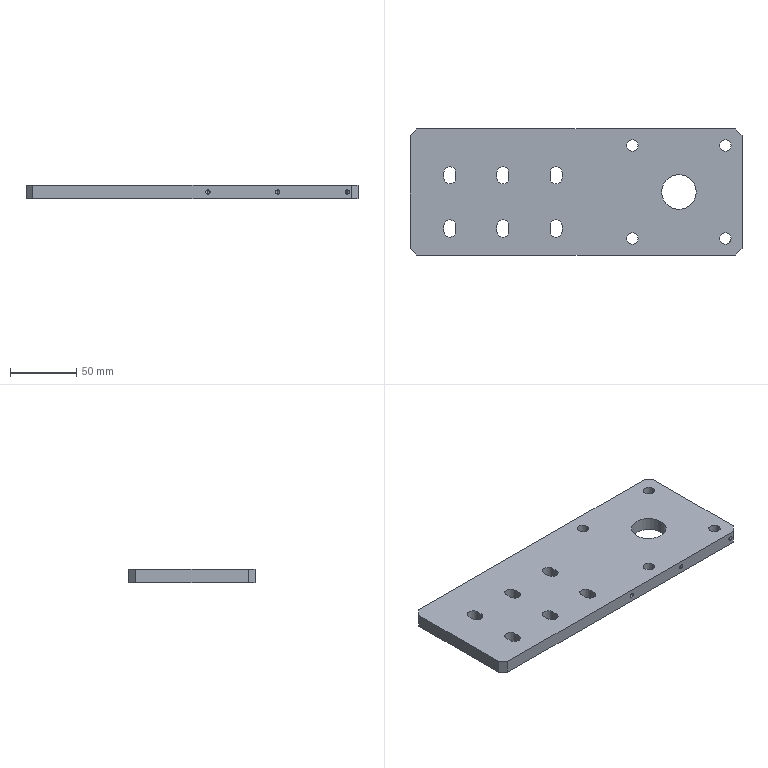Part | SolidWorks | features 3DProfileFeature 4, HoleWzd 4, ICE 2, LPattern 2, Chamfer 1, Extrusion 1 | 1 solid | 56 faces | box 250 x 95 x 10 mm | volume 223177 mm3 | cylinder 28 | plane 22 | cone 6 | commonest cylinder face diameters 9 x12 8.5 x8 3.3 x6 26 x2